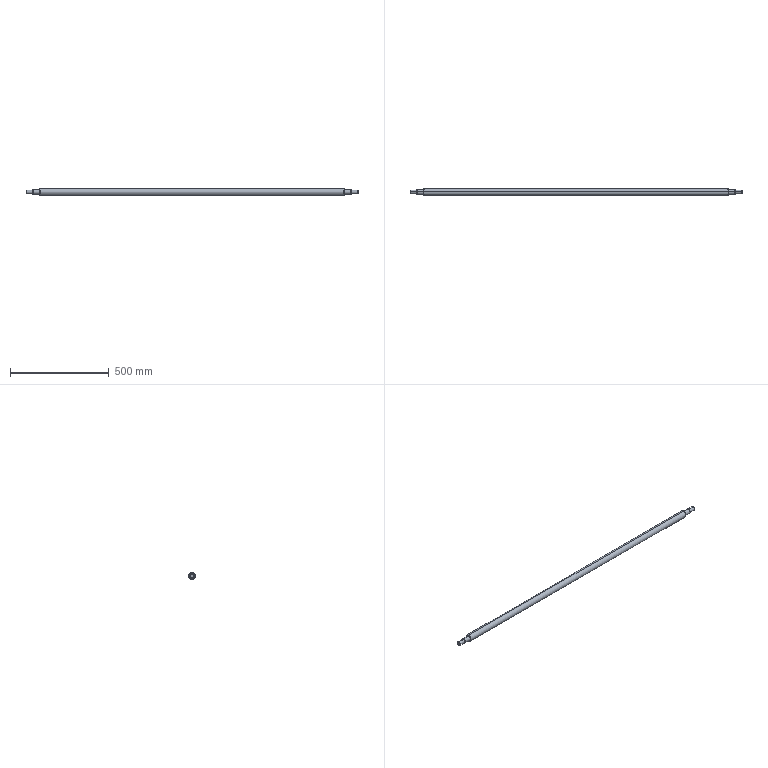Part | STEP file | Microwave Drying Flat Conveyor-CN2500x400-108-101 | 1 solid | 28 faces | box 1682 x 35 x 35 mm | volume 1539685 mm3 | cone 12 | cylinder 10 | plane 6 | commonest cylinder face diameters 20 x4 25 x4 35 x2
STEP:
#1=CARTESIAN_POINT('',(841.,0.,-9.));
#2=VERTEX_POINT('',#1);
#3=CARTESIAN_POINT('',(841.,0.,9.));
#4=VERTEX_POINT('',#3);
#5=CARTESIAN_POINT('',(841.,0.,0.));
#6=DIRECTION('',(1.,0.,0.));
#7=DIRECTION('',(0.,0.,1.));
#8=AXIS2_PLACEMENT_3D('',#5,#6,#7);
#9=CIRCLE('',#8,9.);
#10=EDGE_CURVE('',#2,#4,#9,.T.);
#11=ORIENTED_EDGE('',*,*,#10,.F.);
#12=CARTESIAN_POINT('',(840.,0.,-10.));
#13=VERTEX_POINT('',#12);
#14=CARTESIAN_POINT('',(840.,0.,-10.));
#15=DIRECTION('',(-0.7071,0.,-0.7071));
#16=VECTOR('',#15,1000.);
#17=LINE('',#14,#16);
#18=EDGE_CURVE('',#2,#13,#17,.T.);
#19=ORIENTED_EDGE('',*,*,#18,.T.);
#20=CARTESIAN_POINT('',(840.,0.,10.));
#21=VERTEX_POINT('',#20);
#22=CARTESIAN_POINT('',(840.,0.,0.));
#23=DIRECTION('',(-1.,0.,0.));
#24=DIRECTION('',(0.,0.,1.));
#25=AXIS2_PLACEMENT_3D('',#22,#23,#24);
#26=CIRCLE('',#25,10.);
#27=EDGE_CURVE('',#21,#13,#26,.T.);
#28=ORIENTED_EDGE('',*,*,#27,.F.);
#29=CARTESIAN_POINT('',(840.,0.,10.));
#30=DIRECTION('',(-0.7071,0.,0.7071));
#31=VECTOR('',#30,1000.);
#32=LINE('',#29,#31);
#33=EDGE_CURVE('',#4,#21,#32,.T.);
#34=ORIENTED_EDGE('',*,*,#33,.F.);
#35=EDGE_LOOP('',(#11,#19,#28,#34));
#36=FACE_OUTER_BOUND('',#35,.T.);
#37=CARTESIAN_POINT('',(840.,0.,0.));
#38=DIRECTION('',(-1.,0.,0.));
#39=DIRECTION('',(0.,0.,1.));
#40=AXIS2_PLACEMENT_3D('',#37,#38,#39);
#41=CONICAL_SURFACE('',#40,10.,0.7854);
#42=ADVANCED_FACE('',(#36),#41,.T.);
#43=CARTESIAN_POINT('',(806.,0.,-11.5));
#44=VERTEX_POINT('',#43);
#45=CARTESIAN_POINT('',(806.,0.,11.5));
#46=VERTEX_POINT('',#45);
#47=CARTESIAN_POINT('',(806.,0.,0.));
#48=DIRECTION('',(1.,0.,0.));
#49=DIRECTION('',(0.,0.,1.));
#50=AXIS2_PLACEMENT_3D('',#47,#48,#49);
#51=CIRCLE('',#50,11.5);
#52=EDGE_CURVE('',#44,#46,#51,.T.);
#53=ORIENTED_EDGE('',*,*,#52,.F.);
#54=CARTESIAN_POINT('',(805.,0.,-12.5));
#55=VERTEX_POINT('',#54);
#56=CARTESIAN_POINT('',(805.,0.,-12.5));
#57=DIRECTION('',(-0.7071,0.,-0.7071));
#58=VECTOR('',#57,1000.);
#59=LINE('',#56,#58);
#60=EDGE_CURVE('',#44,#55,#59,.T.);
#61=ORIENTED_EDGE('',*,*,#60,.T.);
#62=CARTESIAN_POINT('',(805.,0.,12.5));
#63=VERTEX_POINT('',#62);
#64=CARTESIAN_POINT('',(805.,0.,0.));
#65=DIRECTION('',(-1.,0.,0.));
#66=DIRECTION('',(0.,0.,1.));
#67=AXIS2_PLACEMENT_3D('',#64,#65,#66);
#68=CIRCLE('',#67,12.5);
#69=EDGE_CURVE('',#63,#55,#68,.T.);
#70=ORIENTED_EDGE('',*,*,#69,.F.);
#71=CARTESIAN_POINT('',(805.,0.,12.5));
#72=DIRECTION('',(-0.7071,0.,0.7071));
#73=VECTOR('',#72,1000.);
#74=LINE('',#71,#73);
#75=EDGE_CURVE('',#46,#63,#74,.T.);
#76=ORIENTED_EDGE('',*,*,#75,.F.);
#77=EDGE_LOOP('',(#53,#61,#70,#76));
#78=FACE_OUTER_BOUND('',#77,.T.);
#79=CARTESIAN_POINT('',(805.,0.,0.));
#80=DIRECTION('',(-1.,0.,0.));
#81=DIRECTION('',(0.,0.,1.));
#82=AXIS2_PLACEMENT_3D('',#79,#80,#81);
#83=CONICAL_SURFACE('',#82,12.5,0.7854);
#84=ADVANCED_FACE('',(#78),#83,.T.);
#85=CARTESIAN_POINT('',(771.,0.,-16.5));
#86=VERTEX_POINT('',#85);
#87=CARTESIAN_POINT('',(771.,0.,16.5));
#88=VERTEX_POINT('',#87);
#89=CARTESIAN_POINT('',(771.,0.,0.));
#90=DIRECTION('',(1.,0.,0.));
#91=DIRECTION('',(0.,0.,1.));
#92=AXIS2_PLACEMENT_3D('',#89,#90,#91);
#93=CIRCLE('',#92,16.5);
#94=EDGE_CURVE('',#86,#88,#93,.T.);
#95=ORIENTED_EDGE('',*,*,#94,.F.);
#96=CARTESIAN_POINT('',(770.,0.,-17.5));
#97=VERTEX_POINT('',#96);
#98=CARTESIAN_POINT('',(770.,0.,-17.5));
#99=DIRECTION('',(-0.7071,0.,-0.7071));
#100=VECTOR('',#99,1000.);
#101=LINE('',#98,#100);
#102=EDGE_CURVE('',#86,#97,#101,.T.);
#103=ORIENTED_EDGE('',*,*,#102,.T.);
#104=CARTESIAN_POINT('',(770.,0.,17.5));
#105=VERTEX_POINT('',#104);
#106=CARTESIAN_POINT('',(770.,0.,0.));
#107=DIRECTION('',(-1.,0.,0.));
#108=DIRECTION('',(0.,0.,1.));
#109=AXIS2_PLACEMENT_3D('',#106,#107,#108);
#110=CIRCLE('',#109,17.5);
#111=EDGE_CURVE('',#105,#97,#110,.T.);
#112=ORIENTED_EDGE('',*,*,#111,.F.);
#113=CARTESIAN_POINT('',(770.,0.,17.5));
#114=DIRECTION('',(-0.7071,0.,0.7071));
#115=VECTOR('',#114,1000.);
#116=LINE('',#113,#115);
#117=EDGE_CURVE('',#88,#105,#116,.T.);
#118=ORIENTED_EDGE('',*,*,#117,.F.);
#119=EDGE_LOOP('',(#95,#103,#112,#118));
#120=FACE_OUTER_BOUND('',#119,.T.);
#121=CARTESIAN_POINT('',(770.,0.,0.));
#122=DIRECTION('',(-1.,0.,0.));
#123=DIRECTION('',(0.,0.,1.));
#124=AXIS2_PLACEMENT_3D('',#121,#122,#123);
#125=CONICAL_SURFACE('',#124,17.5,0.7854);
#126=ADVANCED_FACE('',(#120),#125,.T.);
#127=CARTESIAN_POINT('',(-771.,0.,16.5));
#128=VERTEX_POINT('',#127);
#129=CARTESIAN_POINT('',(-771.,0.,-16.5));
#130=VERTEX_POINT('',#129);
#131=CARTESIAN_POINT('',(-771.,0.,0.));
#132=DIRECTION('',(-1.,0.,0.));
#133=DIRECTION('',(0.,0.,-1.));
#134=AXIS2_PLACEMENT_3D('',#131,#132,#133);
#135=CIRCLE('',#134,16.5);
#136=EDGE_CURVE('',#128,#130,#135,.T.);
#137=ORIENTED_EDGE('',*,*,#136,.F.);
#138=CARTESIAN_POINT('',(-770.,0.,17.5));
#139=VERTEX_POINT('',#138);
#140=CARTESIAN_POINT('',(-771.,0.,16.5));
#141=DIRECTION('',(0.7071,0.,0.7071));
#142=VECTOR('',#141,1000.);
#143=LINE('',#140,#142);
#144=EDGE_CURVE('',#128,#139,#143,.T.);
#145=ORIENTED_EDGE('',*,*,#144,.T.);
#146=CARTESIAN_POINT('',(-770.,0.,-17.5));
#147=VERTEX_POINT('',#146);
#148=CARTESIAN_POINT('',(-770.,0.,0.));
#149=DIRECTION('',(1.,0.,0.));
#150=DIRECTION('',(0.,0.,-1.));
#151=AXIS2_PLACEMENT_3D('',#148,#149,#150);
#152=CIRCLE('',#151,17.5);
#153=EDGE_CURVE('',#147,#139,#152,.T.);
#154=ORIENTED_EDGE('',*,*,#153,.F.);
#155=CARTESIAN_POINT('',(-771.,0.,-16.5));
#156=DIRECTION('',(0.7071,0.,-0.7071));
#157=VECTOR('',#156,1000.);
#158=LINE('',#155,#157);
#159=EDGE_CURVE('',#130,#147,#158,.T.);
#160=ORIENTED_EDGE('',*,*,#159,.F.);
#161=EDGE_LOOP('',(#137,#145,#154,#160));
#162=FACE_OUTER_BOUND('',#161,.T.);
#163=CARTESIAN_POINT('',(-771.,0.,0.));
#164=DIRECTION('',(1.,0.,0.));
#165=DIRECTION('',(0.,0.,-1.));
#166=AXIS2_PLACEMENT_3D('',#163,#164,#165);
#167=CONICAL_SURFACE('',#166,16.5,0.7854);
#168=ADVANCED_FACE('',(#162),#167,.T.);
#169=CARTESIAN_POINT('',(-806.,0.,11.5));
#170=VERTEX_POINT('',#169);
#171=CARTESIAN_POINT('',(-806.,0.,-11.5));
#172=VERTEX_POINT('',#171);
#173=CARTESIAN_POINT('',(-806.,0.,0.));
#174=DIRECTION('',(-1.,0.,0.));
#175=DIRECTION('',(0.,0.,-1.));
#176=AXIS2_PLACEMENT_3D('',#173,#174,#175);
#177=CIRCLE('',#176,11.5);
#178=EDGE_CURVE('',#170,#172,#177,.T.);
#179=ORIENTED_EDGE('',*,*,#178,.F.);
#180=CARTESIAN_POINT('',(-805.,0.,12.5));
#181=VERTEX_POINT('',#180);
#182=CARTESIAN_POINT('',(-806.,0.,11.5));
#183=DIRECTION('',(0.7071,0.,0.7071));
#184=VECTOR('',#183,1000.);
#185=LINE('',#182,#184);
#186=EDGE_CURVE('',#170,#181,#185,.T.);
#187=ORIENTED_EDGE('',*,*,#186,.T.);
#188=CARTESIAN_POINT('',(-805.,0.,-12.5));
#189=VERTEX_POINT('',#188);
#190=CARTESIAN_POINT('',(-805.,0.,0.));
#191=DIRECTION('',(1.,0.,0.));
#192=DIRECTION('',(0.,0.,-1.));
#193=AXIS2_PLACEMENT_3D('',#190,#191,#192);
#194=CIRCLE('',#193,12.5);
#195=EDGE_CURVE('',#189,#181,#194,.T.);
#196=ORIENTED_EDGE('',*,*,#195,.F.);
#197=CARTESIAN_POINT('',(-806.,0.,-11.5));
#198=DIRECTION('',(0.7071,0.,-0.7071));
#199=VECTOR('',#198,1000.);
#200=LINE('',#197,#199);
#201=EDGE_CURVE('',#172,#189,#200,.T.);
#202=ORIENTED_EDGE('',*,*,#201,.F.);
#203=EDGE_LOOP('',(#179,#187,#196,#202));
#204=FACE_OUTER_BOUND('',#203,.T.);
#205=CARTESIAN_POINT('',(-806.,0.,0.));
#206=DIRECTION('',(1.,0.,0.));
#207=DIRECTION('',(0.,0.,-1.));
#208=AXIS2_PLACEMENT_3D('',#205,#206,#207);
#209=CONICAL_SURFACE('',#208,11.5,0.7854);
#210=ADVANCED_FACE('',(#204),#209,.T.);
#211=CARTESIAN_POINT('',(-841.,0.,9.));
#212=VERTEX_POINT('',#211);
#213=CARTESIAN_POINT('',(-841.,0.,-9.));
#214=VERTEX_POINT('',#213);
#215=CARTESIAN_POINT('',(-841.,0.,0.));
#216=DIRECTION('',(-1.,0.,0.));
#217=DIRECTION('',(0.,0.,-1.));
#218=AXIS2_PLACEMENT_3D('',#215,#216,#217);
#219=CIRCLE('',#218,9.);
#220=EDGE_CURVE('',#212,#214,#219,.T.);
#221=ORIENTED_EDGE('',*,*,#220,.F.);
#222=CARTESIAN_POINT('',(-840.,0.,10.));
#223=VERTEX_POINT('',#222);
#224=CARTESIAN_POINT('',(-841.,0.,9.));
#225=DIRECTION('',(0.7071,0.,0.7071));
#226=VECTOR('',#225,1000.);
#227=LINE('',#224,#226);
#228=EDGE_CURVE('',#212,#223,#227,.T.);
#229=ORIENTED_EDGE('',*,*,#228,.T.);
#230=CARTESIAN_POINT('',(-840.,0.,-10.));
#231=VERTEX_POINT('',#230);
#232=CARTESIAN_POINT('',(-840.,0.,0.));
#233=DIRECTION('',(1.,0.,0.));
#234=DIRECTION('',(0.,0.,-1.));
#235=AXIS2_PLACEMENT_3D('',#232,#233,#234);
#236=CIRCLE('',#235,10.);
#237=EDGE_CURVE('',#231,#223,#236,.T.);
#238=ORIENTED_EDGE('',*,*,#237,.F.);
#239=CARTESIAN_POINT('',(-841.,0.,-9.));
#240=DIRECTION('',(0.7071,0.,-0.7071));
#241=VECTOR('',#240,1000.);
#242=LINE('',#239,#241);
#243=EDGE_CURVE('',#214,#231,#242,.T.);
#244=ORIENTED_EDGE('',*,*,#243,.F.);
#245=EDGE_LOOP('',(#221,#229,#238,#244));
#246=FACE_OUTER_BOUND('',#245,.T.);
#247=CARTESIAN_POINT('',(-841.,0.,0.));
#248=DIRECTION('',(1.,0.,0.));
#249=DIRECTION('',(0.,0.,-1.));
#250=AXIS2_PLACEMENT_3D('',#247,#248,#249);
#251=CONICAL_SURFACE('',#250,9.,0.7854);
#252=ADVANCED_FACE('',(#246),#251,.T.);
#253=ORIENTED_EDGE('',*,*,#27,.T.);
#254=CARTESIAN_POINT('',(806.,0.,-10.));
#255=VERTEX_POINT('',#254);
#256=CARTESIAN_POINT('',(-209.5,0.,-10.));
#257=DIRECTION('',(-1.,0.,0.));
#258=VECTOR('',#257,1000.);
#259=LINE('',#256,#258);
#260=EDGE_CURVE('',#13,#255,#259,.T.);
#261=ORIENTED_EDGE('',*,*,#260,.T.);
#262=CARTESIAN_POINT('',(806.,0.,10.));
#263=VERTEX_POINT('',#262);
#264=CARTESIAN_POINT('',(806.,0.,0.));
#265=DIRECTION('',(-1.,0.,0.));
#266=DIRECTION('',(0.,0.,1.));
#267=AXIS2_PLACEMENT_3D('',#264,#265,#266);
#268=CIRCLE('',#267,10.);
#269=EDGE_CURVE('',#263,#255,#268,.T.);
#270=ORIENTED_EDGE('',*,*,#269,.F.);
#271=CARTESIAN_POINT('',(-209.5,0.,10.));
#272=DIRECTION('',(-1.,0.,0.));
#273=VECTOR('',#272,1000.);
#274=LINE('',#271,#273);
#275=EDGE_CURVE('',#21,#263,#274,.T.);
#276=ORIENTED_EDGE('',*,*,#275,.F.);
#277=EDGE_LOOP('',(#253,#261,#270,#276));
#278=FACE_OUTER_BOUND('',#277,.T.);
#279=CARTESIAN_POINT('',(-209.5,0.,0.));
#280=DIRECTION('',(-1.,0.,0.));
#281=DIRECTION('',(0.,0.,1.));
#282=AXIS2_PLACEMENT_3D('',#279,#280,#281);
#283=CYLINDRICAL_SURFACE('',#282,10.);
#284=ADVANCED_FACE('',(#278),#283,.T.);
#285=ORIENTED_EDGE('',*,*,#69,.T.);
#286=CARTESIAN_POINT('',(771.,0.,-12.5));
#287=VERTEX_POINT('',#286);
#288=CARTESIAN_POINT('',(-209.5,0.,-12.5));
#289=DIRECTION('',(-1.,0.,0.));
#290=VECTOR('',#289,1000.);
#291=LINE('',#288,#290);
#292=EDGE_CURVE('',#55,#287,#291,.T.);
#293=ORIENTED_EDGE('',*,*,#292,.T.);
#294=CARTESIAN_POINT('',(771.,0.,12.5));
#295=VERTEX_POINT('',#294);
#296=CARTESIAN_POINT('',(771.,0.,0.));
#297=DIRECTION('',(-1.,0.,0.));
#298=DIRECTION('',(0.,0.,1.));
#299=AXIS2_PLACEMENT_3D('',#296,#297,#298);
#300=CIRCLE('',#299,12.5);
#301=EDGE_CURVE('',#295,#287,#300,.T.);
#302=ORIENTED_EDGE('',*,*,#301,.F.);
#303=CARTESIAN_POINT('',(-209.5,0.,12.5));
#304=DIRECTION('',(-1.,0.,0.));
#305=VECTOR('',#304,1000.);
#306=LINE('',#303,#305);
#307=EDGE_CURVE('',#63,#295,#306,.T.);
#308=ORIENTED_EDGE('',*,*,#307,.F.);
#309=EDGE_LOOP('',(#285,#293,#302,#308));
#310=FACE_OUTER_BOUND('',#309,.T.);
#311=CARTESIAN_POINT('',(-209.5,0.,0.));
#312=DIRECTION('',(-1.,0.,0.));
#313=DIRECTION('',(0.,0.,1.));
#314=AXIS2_PLACEMENT_3D('',#311,#312,#313);
#315=CYLINDRICAL_SURFACE('',#314,12.5);
#316=ADVANCED_FACE('',(#310),#315,.T.);
#317=ORIENTED_EDGE('',*,*,#111,.T.);
#318=CARTESIAN_POINT('',(-209.5,0.,-17.5));
#319=DIRECTION('',(-1.,0.,0.));
#320=VECTOR('',#319,1000.);
#321=LINE('',#318,#320);
#322=EDGE_CURVE('',#97,#147,#321,.T.);
#323=ORIENTED_EDGE('',*,*,#322,.T.);
#324=ORIENTED_EDGE('',*,*,#153,.T.);
#325=CARTESIAN_POINT('',(-209.5,0.,17.5));
#326=DIRECTION('',(-1.,0.,0.));
#327=VECTOR('',#326,1000.);
#328=LINE('',#325,#327);
#329=EDGE_CURVE('',#105,#139,#328,.T.);
#330=ORIENTED_EDGE('',*,*,#329,.F.);
#331=EDGE_LOOP('',(#317,#323,#324,#330));
#332=FACE_OUTER_BOUND('',#331,.T.);
#333=CARTESIAN_POINT('',(-209.5,0.,0.));
#334=DIRECTION('',(-1.,0.,0.));
#335=DIRECTION('',(0.,0.,1.));
#336=AXIS2_PLACEMENT_3D('',#333,#334,#335);
#337=CYLINDRICAL_SURFACE('',#336,17.5);
#338=ADVANCED_FACE('',(#332),#337,.T.);
#339=CARTESIAN_POINT('',(-771.,0.,12.5));
#340=VERTEX_POINT('',#339);
#341=CARTESIAN_POINT('',(-771.,0.,-12.5));
#342=VERTEX_POINT('',#341);
#343=CARTESIAN_POINT('',(-771.,0.,0.));
#344=DIRECTION('',(-1.,0.,0.));
#345=DIRECTION('',(0.,0.,1.));
#346=AXIS2_PLACEMENT_3D('',#343,#344,#345);
#347=CIRCLE('',#346,12.5);
#348=EDGE_CURVE('',#340,#342,#347,.T.);
#349=ORIENTED_EDGE('',*,*,#348,.T.);
#350=CARTESIAN_POINT('',(-209.5,0.,-12.5));
#351=DIRECTION('',(-1.,0.,0.));
#352=VECTOR('',#351,1000.);
#353=LINE('',#350,#352);
#354=EDGE_CURVE('',#342,#189,#353,.T.);
#355=ORIENTED_EDGE('',*,*,#354,.T.);
#356=ORIENTED_EDGE('',*,*,#195,.T.);
#357=CARTESIAN_POINT('',(-209.5,0.,12.5));
#358=DIRECTION('',(-1.,0.,0.));
#359=VECTOR('',#358,1000.);
#360=LINE('',#357,#359);
#361=EDGE_CURVE('',#340,#181,#360,.T.);
#362=ORIENTED_EDGE('',*,*,#361,.F.);
#363=EDGE_LOOP('',(#349,#355,#356,#362));
#364=FACE_OUTER_BOUND('',#363,.T.);
#365=CARTESIAN_POINT('',(-209.5,0.,0.));
#366=DIRECTION('',(-1.,0.,0.));
#367=DIRECTION('',(0.,0.,1.));
#368=AXIS2_PLACEMENT_3D('',#365,#366,#367);
#369=CYLINDRICAL_SURFACE('',#368,12.5);
#370=ADVANCED_FACE('',(#364),#369,.T.);
#371=CARTESIAN_POINT('',(-806.,0.,10.));
#372=VERTEX_POINT('',#371);
#373=CARTESIAN_POINT('',(-806.,0.,-10.));
#374=VERTEX_POINT('',#373);
#375=CARTESIAN_POINT('',(-806.,0.,0.));
#376=DIRECTION('',(-1.,0.,0.));
#377=DIRECTION('',(0.,0.,1.));
#378=AXIS2_PLACEMENT_3D('',#375,#376,#377);
#379=CIRCLE('',#378,10.);
#380=EDGE_CURVE('',#372,#374,#379,.T.);
#381=ORIENTED_EDGE('',*,*,#380,.T.);
#382=CARTESIAN_POINT('',(-209.5,0.,-10.));
#383=DIRECTION('',(-1.,0.,0.));
#384=VECTOR('',#383,1000.);
#385=LINE('',#382,#384);
#386=EDGE_CURVE('',#374,#231,#385,.T.);
#387=ORIENTED_EDGE('',*,*,#386,.T.);
#388=ORIENTED_EDGE('',*,*,#237,.T.);
#389=CARTESIAN_POINT('',(-209.5,0.,10.));
#390=DIRECTION('',(-1.,0.,0.));
#391=VECTOR('',#390,1000.);
#392=LINE('',#389,#391);
#393=EDGE_CURVE('',#372,#223,#392,.T.);
#394=ORIENTED_EDGE('',*,*,#393,.F.);
#395=EDGE_LOOP('',(#381,#387,#388,#394));
#396=FACE_OUTER_BOUND('',#395,.T.);
#397=CARTESIAN_POINT('',(-209.5,0.,0.));
#398=DIRECTION('',(-1.,0.,0.));
#399=DIRECTION('',(0.,0.,1.));
#400=AXIS2_PLACEMENT_3D('',#397,#398,#399);
#401=CYLINDRICAL_SURFACE('',#400,10.);
#402=ADVANCED_FACE('',(#396),#401,.T.);
#403=CARTESIAN_POINT('',(-841.,0.,0.));
#404=DIRECTION('',(-1.,0.,0.));
#405=DIRECTION('',(0.,0.,-1.));
#406=AXIS2_PLACEMENT_3D('',#403,#404,#405);
#407=CIRCLE('',#406,9.);
#408=EDGE_CURVE('',#214,#212,#407,.T.);
#409=ORIENTED_EDGE('',*,*,#408,.T.);
#410=ORIENTED_EDGE('',*,*,#220,.T.);
#411=EDGE_LOOP('',(#409,#410));
#412=FACE_OUTER_BOUND('',#411,.T.);
#413=CARTESIAN_POINT('',(-841.,10.,0.));
#414=DIRECTION('',(1.,0.,0.));
#415=DIRECTION('',(0.,0.,-1.));
#416=AXIS2_PLACEMENT_3D('',#413,#414,#415);
#417=PLANE('',#416);
#418=ADVANCED_FACE('',(#412),#417,.F.);
#419=ORIENTED_EDGE('',*,*,#386,.F.);
#420=CARTESIAN_POINT('',(-806.,0.,0.));
#421=DIRECTION('',(-1.,0.,0.));
#422=DIRECTION('',(0.,0.,1.));
#423=AXIS2_PLACEMENT_3D('',#420,#421,#422);
#424=CIRCLE('',#423,10.);
#425=EDGE_CURVE('',#374,#372,#424,.T.);
#426=ORIENTED_EDGE('',*,*,#425,.T.);
#427=ORIENTED_EDGE('',*,*,#393,.T.);
#428=CARTESIAN_POINT('',(-840.,0.,0.));
#429=DIRECTION('',(1.,0.,0.));
#430=DIRECTION('',(0.,0.,-1.));
#431=AXIS2_PLACEMENT_3D('',#428,#429,#430);
#432=CIRCLE('',#431,10.);
#433=EDGE_CURVE('',#223,#231,#432,.T.);
#434=ORIENTED_EDGE('',*,*,#433,.T.);
#435=EDGE_LOOP('',(#419,#426,#427,#434));
#436=FACE_OUTER_BOUND('',#435,.T.);
#437=CARTESIAN_POINT('',(-209.5,0.,0.));
#438=DIRECTION('',(-1.,0.,0.));
#439=DIRECTION('',(0.,0.,1.));
#440=AXIS2_PLACEMENT_3D('',#437,#438,#439);
#441=CYLINDRICAL_SURFACE('',#440,10.);
#442=ADVANCED_FACE('',(#436),#441,.T.);
#443=CARTESIAN_POINT('',(-806.,0.,0.));
#444=DIRECTION('',(-1.,0.,0.));
#445=DIRECTION('',(0.,0.,-1.));
#446=AXIS2_PLACEMENT_3D('',#443,#444,#445);
#447=CIRCLE('',#446,11.5);
#448=EDGE_CURVE('',#172,#170,#447,.T.);
#449=ORIENTED_EDGE('',*,*,#448,.T.);
#450=ORIENTED_EDGE('',*,*,#178,.T.);
#451=EDGE_LOOP('',(#449,#450));
#452=FACE_OUTER_BOUND('',#451,.T.);
#453=ORIENTED_EDGE('',*,*,#380,.F.);
#454=ORIENTED_EDGE('',*,*,#425,.F.);
#455=EDGE_LOOP('',(#453,#454));
#456=FACE_BOUND('',#455,.T.);
#457=CARTESIAN_POINT('',(-806.,12.5,0.));
#458=DIRECTION('',(1.,0.,0.));
#459=DIRECTION('',(0.,0.,-1.));
#460=AXIS2_PLACEMENT_3D('',#457,#458,#459);
#461=PLANE('',#460);
#462=ADVANCED_FACE('',(#452,#456),#461,.F.);
#463=ORIENTED_EDGE('',*,*,#354,.F.);
#464=CARTESIAN_POINT('',(-771.,0.,0.));
#465=DIRECTION('',(-1.,0.,0.));
#466=DIRECTION('',(0.,0.,1.));
#467=AXIS2_PLACEMENT_3D('',#464,#465,#466);
#468=CIRCLE('',#467,12.5);
#469=EDGE_CURVE('',#342,#340,#468,.T.);
#470=ORIENTED_EDGE('',*,*,#469,.T.);
#471=ORIENTED_EDGE('',*,*,#361,.T.);
#472=CARTESIAN_POINT('',(-805.,0.,0.));
#473=DIRECTION('',(1.,0.,0.));
#474=DIRECTION('',(0.,0.,-1.));
#475=AXIS2_PLACEMENT_3D('',#472,#473,#474);
#476=CIRCLE('',#475,12.5);
#477=EDGE_CURVE('',#181,#189,#476,.T.);
#478=ORIENTED_EDGE('',*,*,#477,.T.);
#479=EDGE_LOOP('',(#463,#470,#471,#478));
#480=FACE_OUTER_BOUND('',#479,.T.);
#481=CARTESIAN_POINT('',(-209.5,0.,0.));
#482=DIRECTION('',(-1.,0.,0.));
#483=DIRECTION('',(0.,0.,1.));
#484=AXIS2_PLACEMENT_3D('',#481,#482,#483);
#485=CYLINDRICAL_SURFACE('',#484,12.5);
#486=ADVANCED_FACE('',(#480),#485,.T.);
#487=CARTESIAN_POINT('',(-771.,0.,0.));
#488=DIRECTION('',(-1.,0.,0.));
#489=DIRECTION('',(0.,0.,-1.));
#490=AXIS2_PLACEMENT_3D('',#487,#488,#489);
#491=CIRCLE('',#490,16.5);
#492=EDGE_CURVE('',#130,#128,#491,.T.);
#493=ORIENTED_EDGE('',*,*,#492,.T.);
#494=ORIENTED_EDGE('',*,*,#136,.T.);
#495=EDGE_LOOP('',(#493,#494));
#496=FACE_OUTER_BOUND('',#495,.T.);
#497=ORIENTED_EDGE('',*,*,#348,.F.);
#498=ORIENTED_EDGE('',*,*,#469,.F.);
#499=EDGE_LOOP('',(#497,#498));
#500=FACE_BOUND('',#499,.T.);
#501=CARTESIAN_POINT('',(-771.,17.5,0.));
#502=DIRECTION('',(1.,0.,0.));
#503=DIRECTION('',(0.,0.,-1.));
#504=AXIS2_PLACEMENT_3D('',#501,#502,#503);
#505=PLANE('',#504);
#506=ADVANCED_FACE('',(#496,#500),#505,.F.);
#507=ORIENTED_EDGE('',*,*,#322,.F.);
#508=CARTESIAN_POINT('',(770.,0.,0.));
#509=DIRECTION('',(-1.,0.,0.));
#510=DIRECTION('',(0.,0.,1.));
#511=AXIS2_PLACEMENT_3D('',#508,#509,#510);
#512=CIRCLE('',#511,17.5);
#513=EDGE_CURVE('',#97,#105,#512,.T.);
#514=ORIENTED_EDGE('',*,*,#513,.T.);
#515=ORIENTED_EDGE('',*,*,#329,.T.);
#516=CARTESIAN_POINT('',(-770.,0.,0.));
#517=DIRECTION('',(1.,0.,0.));
#518=DIRECTION('',(0.,0.,-1.));
#519=AXIS2_PLACEMENT_3D('',#516,#517,#518);
#520=CIRCLE('',#519,17.5);
#521=EDGE_CURVE('',#139,#147,#520,.T.);
#522=ORIENTED_EDGE('',*,*,#521,.T.);
#523=EDGE_LOOP('',(#507,#514,#515,#522));
#524=FACE_OUTER_BOUND('',#523,.T.);
#525=CARTESIAN_POINT('',(-209.5,0.,0.));
#526=DIRECTION('',(-1.,0.,0.));
#527=DIRECTION('',(0.,0.,1.));
#528=AXIS2_PLACEMENT_3D('',#525,#526,#527);
#529=CYLINDRICAL_SURFACE('',#528,17.5);
#530=ADVANCED_FACE('',(#524),#529,.T.);
#531=CARTESIAN_POINT('',(771.,0.,0.));
#532=DIRECTION('',(1.,0.,0.));
#533=DIRECTION('',(0.,0.,1.));
#534=AXIS2_PLACEMENT_3D('',#531,#532,#533);
#535=CIRCLE('',#534,16.5);
#536=EDGE_CURVE('',#88,#86,#535,.T.);
#537=ORIENTED_EDGE('',*,*,#536,.T.);
#538=ORIENTED_EDGE('',*,*,#94,.T.);
#539=EDGE_LOOP('',(#537,#538));
#540=FACE_OUTER_BOUND('',#539,.T.);
#541=ORIENTED_EDGE('',*,*,#301,.T.);
#542=CARTESIAN_POINT('',(771.,0.,0.));
#543=DIRECTION('',(-1.,0.,0.));
#544=DIRECTION('',(0.,0.,1.));
#545=AXIS2_PLACEMENT_3D('',#542,#543,#544);
#546=CIRCLE('',#545,12.5);
#547=EDGE_CURVE('',#287,#295,#546,.T.);
#548=ORIENTED_EDGE('',*,*,#547,.T.);
#549=EDGE_LOOP('',(#541,#548));
#550=FACE_BOUND('',#549,.T.);
#551=CARTESIAN_POINT('',(771.,12.5,0.));
#552=DIRECTION('',(-1.,0.,0.));
#553=DIRECTION('',(0.,0.,1.));
#554=AXIS2_PLACEMENT_3D('',#551,#552,#553);
#555=PLANE('',#554);
#556=ADVANCED_FACE('',(#540,#550),#555,.F.);
#557=ORIENTED_EDGE('',*,*,#292,.F.);
#558=CARTESIAN_POINT('',(805.,0.,0.));
#559=DIRECTION('',(-1.,0.,0.));
#560=DIRECTION('',(0.,0.,1.));
#561=AXIS2_PLACEMENT_3D('',#558,#559,#560);
#562=CIRCLE('',#561,12.5);
#563=EDGE_CURVE('',#55,#63,#562,.T.);
#564=ORIENTED_EDGE('',*,*,#563,.T.);
#565=ORIENTED_EDGE('',*,*,#307,.T.);
#566=ORIENTED_EDGE('',*,*,#547,.F.);
#567=EDGE_LOOP('',(#557,#564,#565,#566));
#568=FACE_OUTER_BOUND('',#567,.T.);
#569=CARTESIAN_POINT('',(-209.5,0.,0.));
#570=DIRECTION('',(-1.,0.,0.));
#571=DIRECTION('',(0.,0.,1.));
#572=AXIS2_PLACEMENT_3D('',#569,#570,#571);
#573=CYLINDRICAL_SURFACE('',#572,12.5);
#574=ADVANCED_FACE('',(#568),#573,.T.);
#575=CARTESIAN_POINT('',(806.,0.,0.));
#576=DIRECTION('',(1.,0.,0.));
#577=DIRECTION('',(0.,0.,1.));
#578=AXIS2_PLACEMENT_3D('',#575,#576,#577);
#579=CIRCLE('',#578,11.5);
#580=EDGE_CURVE('',#46,#44,#579,.T.);
#581=ORIENTED_EDGE('',*,*,#580,.T.);
#582=ORIENTED_EDGE('',*,*,#52,.T.);
#583=EDGE_LOOP('',(#581,#582));
#584=FACE_OUTER_BOUND('',#583,.T.);
#585=ORIENTED_EDGE('',*,*,#269,.T.);
#586=CARTESIAN_POINT('',(806.,0.,0.));
#587=DIRECTION('',(-1.,0.,0.));
#588=DIRECTION('',(0.,0.,1.));
#589=AXIS2_PLACEMENT_3D('',#586,#587,#588);
#590=CIRCLE('',#589,10.);
#591=EDGE_CURVE('',#255,#263,#590,.T.);
#592=ORIENTED_EDGE('',*,*,#591,.T.);
#593=EDGE_LOOP('',(#585,#592));
#594=FACE_BOUND('',#593,.T.);
#595=CARTESIAN_POINT('',(806.,12.5,0.));
#596=DIRECTION('',(-1.,0.,0.));
#597=DIRECTION('',(0.,0.,1.));
#598=AXIS2_PLACEMENT_3D('',#595,#596,#597);
#599=PLANE('',#598);
#600=ADVANCED_FACE('',(#584,#594),#599,.F.);
#601=ORIENTED_EDGE('',*,*,#260,.F.);
#602=CARTESIAN_POINT('',(840.,0.,0.));
#603=DIRECTION('',(-1.,0.,0.));
#604=DIRECTION('',(0.,0.,1.));
#605=AXIS2_PLACEMENT_3D('',#602,#603,#604);
#606=CIRCLE('',#605,10.);
#607=EDGE_CURVE('',#13,#21,#606,.T.);
#608=ORIENTED_EDGE('',*,*,#607,.T.);
#609=ORIENTED_EDGE('',*,*,#275,.T.);
#610=ORIENTED_EDGE('',*,*,#591,.F.);
#611=EDGE_LOOP('',(#601,#608,#609,#610));
#612=FACE_OUTER_BOUND('',#611,.T.);
#613=CARTESIAN_POINT('',(-209.5,0.,0.));
#614=DIRECTION('',(-1.,0.,0.));
#615=DIRECTION('',(0.,0.,1.));
#616=AXIS2_PLACEMENT_3D('',#613,#614,#615);
#617=CYLINDRICAL_SURFACE('',#616,10.);
#618=ADVANCED_FACE('',(#612),#617,.T.);
#619=CARTESIAN_POINT('',(841.,0.,0.));
#620=DIRECTION('',(1.,0.,0.));
#621=DIRECTION('',(0.,0.,1.));
#622=AXIS2_PLACEMENT_3D('',#619,#620,#621);
#623=CIRCLE('',#622,9.);
#624=EDGE_CURVE('',#4,#2,#623,.T.);
#625=ORIENTED_EDGE('',*,*,#624,.T.);
#626=ORIENTED_EDGE('',*,*,#10,.T.);
#627=EDGE_LOOP('',(#625,#626));
#628=FACE_OUTER_BOUND('',#627,.T.);
#629=CARTESIAN_POINT('',(841.,10.,0.));
#630=DIRECTION('',(-1.,0.,0.));
#631=DIRECTION('',(0.,0.,1.));
#632=AXIS2_PLACEMENT_3D('',#629,#630,#631);
#633=PLANE('',#632);
#634=ADVANCED_FACE('',(#628),#633,.F.);
#635=ORIENTED_EDGE('',*,*,#228,.F.);
#636=ORIENTED_EDGE('',*,*,#408,.F.);
#637=ORIENTED_EDGE('',*,*,#243,.T.);
#638=ORIENTED_EDGE('',*,*,#433,.F.);
#639=EDGE_LOOP('',(#635,#636,#637,#638));
#640=FACE_OUTER_BOUND('',#639,.T.);
#641=CARTESIAN_POINT('',(-841.,0.,0.));
#642=DIRECTION('',(1.,0.,0.));
#643=DIRECTION('',(0.,0.,-1.));
#644=AXIS2_PLACEMENT_3D('',#641,#642,#643);
#645=CONICAL_SURFACE('',#644,9.,0.7854);
#646=ADVANCED_FACE('',(#640),#645,.T.);
#647=ORIENTED_EDGE('',*,*,#186,.F.);
#648=ORIENTED_EDGE('',*,*,#448,.F.);
#649=ORIENTED_EDGE('',*,*,#201,.T.);
#650=ORIENTED_EDGE('',*,*,#477,.F.);
#651=EDGE_LOOP('',(#647,#648,#649,#650));
#652=FACE_OUTER_BOUND('',#651,.T.);
#653=CARTESIAN_POINT('',(-806.,0.,0.));
#654=DIRECTION('',(1.,0.,0.));
#655=DIRECTION('',(0.,0.,-1.));
#656=AXIS2_PLACEMENT_3D('',#653,#654,#655);
#657=CONICAL_SURFACE('',#656,11.5,0.7854);
#658=ADVANCED_FACE('',(#652),#657,.T.);
#659=ORIENTED_EDGE('',*,*,#144,.F.);
#660=ORIENTED_EDGE('',*,*,#492,.F.);
#661=ORIENTED_EDGE('',*,*,#159,.T.);
#662=ORIENTED_EDGE('',*,*,#521,.F.);
#663=EDGE_LOOP('',(#659,#660,#661,#662));
#664=FACE_OUTER_BOUND('',#663,.T.);
#665=CARTESIAN_POINT('',(-771.,0.,0.));
#666=DIRECTION('',(1.,0.,0.));
#667=DIRECTION('',(0.,0.,-1.));
#668=AXIS2_PLACEMENT_3D('',#665,#666,#667);
#669=CONICAL_SURFACE('',#668,16.5,0.7854);
#670=ADVANCED_FACE('',(#664),#669,.T.);
#671=ORIENTED_EDGE('',*,*,#102,.F.);
#672=ORIENTED_EDGE('',*,*,#536,.F.);
#673=ORIENTED_EDGE('',*,*,#117,.T.);
#674=ORIENTED_EDGE('',*,*,#513,.F.);
#675=EDGE_LOOP('',(#671,#672,#673,#674));
#676=FACE_OUTER_BOUND('',#675,.T.);
#677=CARTESIAN_POINT('',(770.,0.,0.));
#678=DIRECTION('',(-1.,0.,0.));
#679=DIRECTION('',(0.,0.,1.));
#680=AXIS2_PLACEMENT_3D('',#677,#678,#679);
#681=CONICAL_SURFACE('',#680,17.5,0.7854);
#682=ADVANCED_FACE('',(#676),#681,.T.);
#683=ORIENTED_EDGE('',*,*,#60,.F.);
#684=ORIENTED_EDGE('',*,*,#580,.F.);
#685=ORIENTED_EDGE('',*,*,#75,.T.);
#686=ORIENTED_EDGE('',*,*,#563,.F.);
#687=EDGE_LOOP('',(#683,#684,#685,#686));
#688=FACE_OUTER_BOUND('',#687,.T.);
#689=CARTESIAN_POINT('',(805.,0.,0.));
#690=DIRECTION('',(-1.,0.,0.));
#691=DIRECTION('',(0.,0.,1.));
#692=AXIS2_PLACEMENT_3D('',#689,#690,#691);
#693=CONICAL_SURFACE('',#692,12.5,0.7854);
#694=ADVANCED_FACE('',(#688),#693,.T.);
#695=ORIENTED_EDGE('',*,*,#18,.F.);
#696=ORIENTED_EDGE('',*,*,#624,.F.);
#697=ORIENTED_EDGE('',*,*,#33,.T.);
#698=ORIENTED_EDGE('',*,*,#607,.F.);
#699=EDGE_LOOP('',(#695,#696,#697,#698));
#700=FACE_OUTER_BOUND('',#699,.T.);
#701=CARTESIAN_POINT('',(840.,0.,0.));
#702=DIRECTION('',(-1.,0.,0.));
#703=DIRECTION('',(0.,0.,1.));
#704=AXIS2_PLACEMENT_3D('',#701,#702,#703);
#705=CONICAL_SURFACE('',#704,10.,0.7854);
#706=ADVANCED_FACE('',(#700),#705,.T.);
#707=CLOSED_SHELL('',(#42,#84,#126,#168,#210,#252,#284,#316,#338,#370,#402,#418,#442,#462,#486,#506,#530,#556,#574,#600,#618,#634,#646,#658,#670,#682,#694,#706));
#708=MANIFOLD_SOLID_BREP('',#707);
#709=CARTESIAN_POINT('',(0.,0.,0.));
#710=DIRECTION('',(0.,0.,1.));
#711=DIRECTION('',(1.,0.,0.));
#712=AXIS2_PLACEMENT_3D('',#709,#710,#711);
#713=(LENGTH_UNIT()NAMED_UNIT(*)SI_UNIT(.MILLI.,.METRE.));
#714=UNCERTAINTY_MEASURE_WITH_UNIT(LENGTH_MEASURE(0.00001),#713,'','');
#715=(NAMED_UNIT(*)PLANE_ANGLE_UNIT()SI_UNIT($,.RADIAN.));
#716=(NAMED_UNIT(*)SI_UNIT($,.STERADIAN.)SOLID_ANGLE_UNIT());
#717=(GEOMETRIC_REPRESENTATION_CONTEXT(3)GLOBAL_UNCERTAINTY_ASSIGNED_CONTEXT((#714))GLOBAL_UNIT_ASSIGNED_CONTEXT((#713,#715,#716))REPRESENTATION_CONTEXT('',''));
#718=ADVANCED_BREP_SHAPE_REPRESENTATION('',(#708,#712),#717);